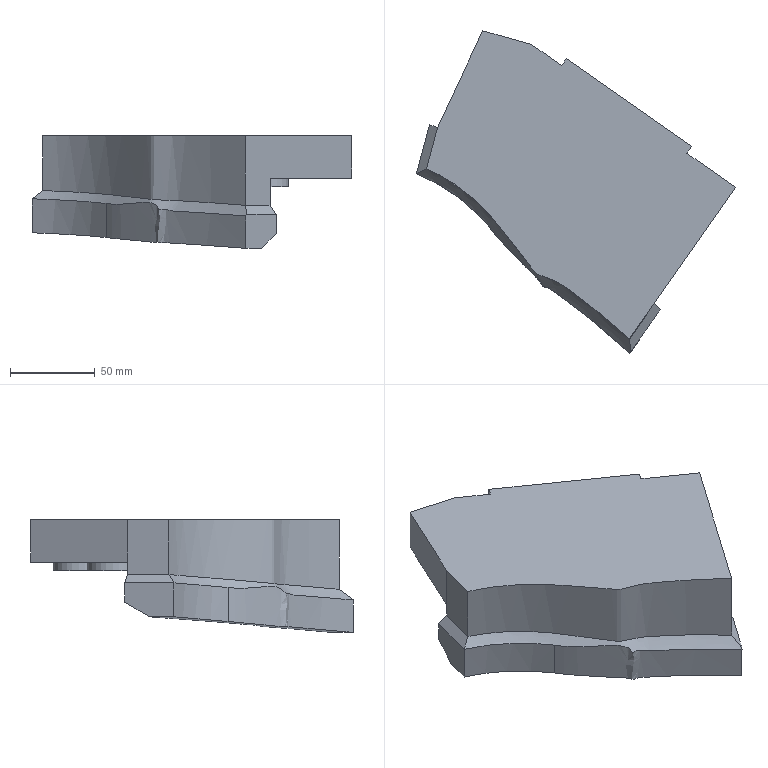Part | NX | features solid 2 | 1 solid | 35 faces | box 187.867 x 189.737 x 66.349 mm | volume 612572 mm3 | plane 20 | spline 10 | cylinder 5 | commonest cylinder face diameters 30 x5